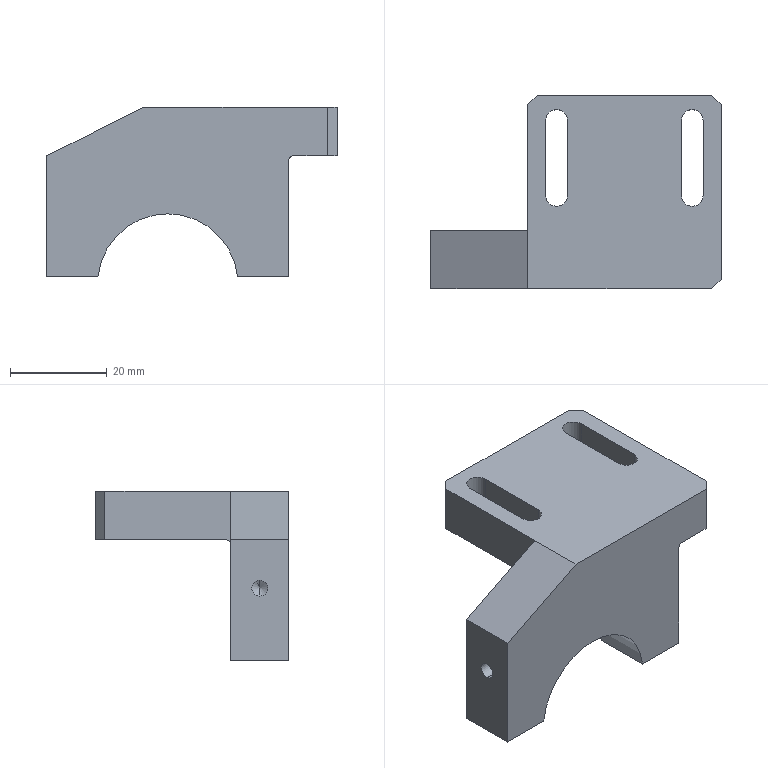Part | 1 solid | 52 faces | box 60 x 40 x 35 mm | volume 25774 mm3 | plane 25 | cylinder 19 | cone 8 | commonest cylinder face diameters 3.3 x8 4.5 x4 8 x4 2 x2 29 x1
STEP:
#1=CARTESIAN_POINT('',(-28.5,-14.,-21.65));
#2=VERTEX_POINT('',#1);
#3=CARTESIAN_POINT('',(-28.5,-14.,-18.35));
#4=VERTEX_POINT('',#3);
#5=CARTESIAN_POINT('',(-28.5,-14.,-20.));
#6=DIRECTION('',(-1.,0.,0.));
#7=DIRECTION('',(0.,0.,1.));
#8=AXIS2_PLACEMENT_3D('',#5,#6,#7);
#9=CIRCLE('',#8,1.65);
#10=EDGE_CURVE('',#2,#4,#9,.T.);
#11=ORIENTED_EDGE('',*,*,#10,.F.);
#12=CARTESIAN_POINT('',(-40.,-14.,-21.65));
#13=VERTEX_POINT('',#12);
#14=CARTESIAN_POINT('',(-40.,-14.,-21.65));
#15=DIRECTION('',(-1.,0.,0.));
#16=VECTOR('',#15,1000.);
#17=LINE('',#14,#16);
#18=EDGE_CURVE('',#13,#2,#17,.F.);
#19=ORIENTED_EDGE('',*,*,#18,.F.);
#20=CARTESIAN_POINT('',(-40.,-14.,-18.35));
#21=VERTEX_POINT('',#20);
#22=CARTESIAN_POINT('',(-40.,-14.,-20.));
#23=DIRECTION('',(-1.,0.,0.));
#24=DIRECTION('',(0.,0.,1.));
#25=AXIS2_PLACEMENT_3D('',#22,#23,#24);
#26=CIRCLE('',#25,1.65);
#27=EDGE_CURVE('',#13,#21,#26,.T.);
#28=ORIENTED_EDGE('',*,*,#27,.T.);
#29=CARTESIAN_POINT('',(-40.,-14.,-18.35));
#30=DIRECTION('',(-1.,0.,0.));
#31=VECTOR('',#30,1000.);
#32=LINE('',#29,#31);
#33=EDGE_CURVE('',#21,#4,#32,.F.);
#34=ORIENTED_EDGE('',*,*,#33,.T.);
#35=EDGE_LOOP('',(#11,#19,#28,#34));
#36=FACE_BOUND('',#35,.T.);
#37=CARTESIAN_POINT('',(-40.,-14.,-20.));
#38=DIRECTION('',(-1.,0.,0.));
#39=DIRECTION('',(0.,0.,-1.));
#40=AXIS2_PLACEMENT_3D('',#37,#38,#39);
#41=CYLINDRICAL_SURFACE('',#40,1.65);
#42=ADVANCED_FACE('',(#36),#41,.F.);
#43=CARTESIAN_POINT('',(-27.509,-14.,-20.));
#44=VERTEX_POINT('',#43);
#45=CARTESIAN_POINT('',(-28.5,-14.,-18.35));
#46=DIRECTION('',(-0.515,0.,0.8572));
#47=VECTOR('',#46,1000.);
#48=LINE('',#45,#47);
#49=EDGE_CURVE('',#4,#44,#48,.F.);
#50=ORIENTED_EDGE('',*,*,#49,.T.);
#51=CARTESIAN_POINT('',(-28.5,-14.,-21.65));
#52=DIRECTION('',(-0.515,0.,-0.8572));
#53=VECTOR('',#52,1000.);
#54=LINE('',#51,#53);
#55=EDGE_CURVE('',#2,#44,#54,.F.);
#56=ORIENTED_EDGE('',*,*,#55,.F.);
#57=ORIENTED_EDGE('',*,*,#10,.T.);
#58=EDGE_LOOP('',(#50,#56,#57));
#59=FACE_BOUND('',#58,.T.);
#60=CARTESIAN_POINT('',(-28.5,-14.,-20.));
#61=DIRECTION('',(-1.,0.,0.));
#62=DIRECTION('',(0.,0.,-1.));
#63=AXIS2_PLACEMENT_3D('',#60,#61,#62);
#64=CONICAL_SURFACE('',#63,1.65,1.03);
#65=ADVANCED_FACE('',(#59),#64,.F.);
#66=CARTESIAN_POINT('',(-1.5,-14.,-18.35));
#67=VERTEX_POINT('',#66);
#68=CARTESIAN_POINT('',(-1.5,-14.,-21.65));
#69=VERTEX_POINT('',#68);
#70=CARTESIAN_POINT('',(-1.5,-14.,-20.));
#71=DIRECTION('',(1.,0.,0.));
#72=DIRECTION('',(0.,0.,-1.));
#73=AXIS2_PLACEMENT_3D('',#70,#71,#72);
#74=CIRCLE('',#73,1.65);
#75=EDGE_CURVE('',#67,#69,#74,.T.);
#76=ORIENTED_EDGE('',*,*,#75,.F.);
#77=CARTESIAN_POINT('',(10.,-14.,-18.35));
#78=VERTEX_POINT('',#77);
#79=CARTESIAN_POINT('',(10.,-14.,-18.35));
#80=DIRECTION('',(1.,0.,0.));
#81=VECTOR('',#80,1000.);
#82=LINE('',#79,#81);
#83=EDGE_CURVE('',#78,#67,#82,.F.);
#84=ORIENTED_EDGE('',*,*,#83,.F.);
#85=CARTESIAN_POINT('',(10.,-14.,-21.65));
#86=VERTEX_POINT('',#85);
#87=CARTESIAN_POINT('',(10.,-14.,-20.));
#88=DIRECTION('',(1.,0.,0.));
#89=DIRECTION('',(0.,0.,-1.));
#90=AXIS2_PLACEMENT_3D('',#87,#88,#89);
#91=CIRCLE('',#90,1.65);
#92=EDGE_CURVE('',#78,#86,#91,.T.);
#93=ORIENTED_EDGE('',*,*,#92,.T.);
#94=CARTESIAN_POINT('',(10.,-14.,-21.65));
#95=DIRECTION('',(1.,0.,0.));
#96=VECTOR('',#95,1000.);
#97=LINE('',#94,#96);
#98=EDGE_CURVE('',#86,#69,#97,.F.);
#99=ORIENTED_EDGE('',*,*,#98,.T.);
#100=EDGE_LOOP('',(#76,#84,#93,#99));
#101=FACE_BOUND('',#100,.T.);
#102=CARTESIAN_POINT('',(10.,-14.,-20.));
#103=DIRECTION('',(1.,0.,0.));
#104=DIRECTION('',(0.,0.,1.));
#105=AXIS2_PLACEMENT_3D('',#102,#103,#104);
#106=CYLINDRICAL_SURFACE('',#105,1.65);
#107=ADVANCED_FACE('',(#101),#106,.F.);
#108=CARTESIAN_POINT('',(-2.491,-14.,-20.));
#109=VERTEX_POINT('',#108);
#110=CARTESIAN_POINT('',(-1.5,-14.,-21.65));
#111=DIRECTION('',(0.515,0.,-0.8572));
#112=VECTOR('',#111,1000.);
#113=LINE('',#110,#112);
#114=EDGE_CURVE('',#69,#109,#113,.F.);
#115=ORIENTED_EDGE('',*,*,#114,.T.);
#116=CARTESIAN_POINT('',(-1.5,-14.,-18.35));
#117=DIRECTION('',(0.515,0.,0.8572));
#118=VECTOR('',#117,1000.);
#119=LINE('',#116,#118);
#120=EDGE_CURVE('',#67,#109,#119,.F.);
#121=ORIENTED_EDGE('',*,*,#120,.F.);
#122=ORIENTED_EDGE('',*,*,#75,.T.);
#123=EDGE_LOOP('',(#115,#121,#122));
#124=FACE_BOUND('',#123,.T.);
#125=CARTESIAN_POINT('',(-1.5,-14.,-20.));
#126=DIRECTION('',(1.,0.,0.));
#127=DIRECTION('',(0.,0.,1.));
#128=AXIS2_PLACEMENT_3D('',#125,#126,#127);
#129=CONICAL_SURFACE('',#128,1.65,1.03);
#130=ADVANCED_FACE('',(#124),#129,.F.);
#131=CARTESIAN_POINT('',(6.65,-14.,-23.5));
#132=VERTEX_POINT('',#131);
#133=CARTESIAN_POINT('',(3.35,-14.,-23.5));
#134=VERTEX_POINT('',#133);
#135=CARTESIAN_POINT('',(5.,-14.,-23.5));
#136=DIRECTION('',(0.,0.,-1.));
#137=DIRECTION('',(-1.,0.,0.));
#138=AXIS2_PLACEMENT_3D('',#135,#136,#137);
#139=CIRCLE('',#138,1.65);
#140=EDGE_CURVE('',#132,#134,#139,.T.);
#141=ORIENTED_EDGE('',*,*,#140,.F.);
#142=CARTESIAN_POINT('',(6.65,-14.,-35.));
#143=VERTEX_POINT('',#142);
#144=CARTESIAN_POINT('',(6.65,-14.,-35.));
#145=DIRECTION('',(0.,0.,-1.));
#146=VECTOR('',#145,1000.);
#147=LINE('',#144,#146);
#148=EDGE_CURVE('',#143,#132,#147,.F.);
#149=ORIENTED_EDGE('',*,*,#148,.F.);
#150=CARTESIAN_POINT('',(3.35,-14.,-35.));
#151=VERTEX_POINT('',#150);
#152=CARTESIAN_POINT('',(5.,-14.,-35.));
#153=DIRECTION('',(0.,0.,-1.));
#154=DIRECTION('',(-1.,0.,0.));
#155=AXIS2_PLACEMENT_3D('',#152,#153,#154);
#156=CIRCLE('',#155,1.65);
#157=EDGE_CURVE('',#143,#151,#156,.T.);
#158=ORIENTED_EDGE('',*,*,#157,.T.);
#159=CARTESIAN_POINT('',(3.35,-14.,-35.));
#160=DIRECTION('',(0.,0.,-1.));
#161=VECTOR('',#160,1000.);
#162=LINE('',#159,#161);
#163=EDGE_CURVE('',#151,#134,#162,.F.);
#164=ORIENTED_EDGE('',*,*,#163,.T.);
#165=EDGE_LOOP('',(#141,#149,#158,#164));
#166=FACE_BOUND('',#165,.T.);
#167=CARTESIAN_POINT('',(5.,-14.,-35.));
#168=DIRECTION('',(0.,0.,-1.));
#169=DIRECTION('',(1.,0.,0.));
#170=AXIS2_PLACEMENT_3D('',#167,#168,#169);
#171=CYLINDRICAL_SURFACE('',#170,1.65);
#172=ADVANCED_FACE('',(#166),#171,.F.);
#173=CARTESIAN_POINT('',(5.,-14.,-22.509));
#174=VERTEX_POINT('',#173);
#175=CARTESIAN_POINT('',(3.35,-14.,-23.5));
#176=DIRECTION('',(-0.8572,0.,-0.515));
#177=VECTOR('',#176,1000.);
#178=LINE('',#175,#177);
#179=EDGE_CURVE('',#134,#174,#178,.F.);
#180=ORIENTED_EDGE('',*,*,#179,.T.);
#181=CARTESIAN_POINT('',(6.65,-14.,-23.5));
#182=DIRECTION('',(0.8572,0.,-0.515));
#183=VECTOR('',#182,1000.);
#184=LINE('',#181,#183);
#185=EDGE_CURVE('',#132,#174,#184,.F.);
#186=ORIENTED_EDGE('',*,*,#185,.F.);
#187=ORIENTED_EDGE('',*,*,#140,.T.);
#188=EDGE_LOOP('',(#180,#186,#187));
#189=FACE_BOUND('',#188,.T.);
#190=CARTESIAN_POINT('',(5.,-14.,-23.5));
#191=DIRECTION('',(0.,0.,-1.));
#192=DIRECTION('',(1.,0.,0.));
#193=AXIS2_PLACEMENT_3D('',#190,#191,#192);
#194=CONICAL_SURFACE('',#193,1.65,1.03);
#195=ADVANCED_FACE('',(#189),#194,.F.);
#196=CARTESIAN_POINT('',(-33.35,-14.,-23.5));
#197=VERTEX_POINT('',#196);
#198=CARTESIAN_POINT('',(-36.65,-14.,-23.5));
#199=VERTEX_POINT('',#198);
#200=CARTESIAN_POINT('',(-35.,-14.,-23.5));
#201=DIRECTION('',(0.,0.,-1.));
#202=DIRECTION('',(-1.,0.,0.));
#203=AXIS2_PLACEMENT_3D('',#200,#201,#202);
#204=CIRCLE('',#203,1.65);
#205=EDGE_CURVE('',#197,#199,#204,.T.);
#206=ORIENTED_EDGE('',*,*,#205,.F.);
#207=CARTESIAN_POINT('',(-33.35,-14.,-35.));
#208=VERTEX_POINT('',#207);
#209=CARTESIAN_POINT('',(-33.35,-14.,-35.));
#210=DIRECTION('',(0.,0.,-1.));
#211=VECTOR('',#210,1000.);
#212=LINE('',#209,#211);
#213=EDGE_CURVE('',#208,#197,#212,.F.);
#214=ORIENTED_EDGE('',*,*,#213,.F.);
#215=CARTESIAN_POINT('',(-36.65,-14.,-35.));
#216=VERTEX_POINT('',#215);
#217=CARTESIAN_POINT('',(-35.,-14.,-35.));
#218=DIRECTION('',(0.,0.,-1.));
#219=DIRECTION('',(-1.,0.,0.));
#220=AXIS2_PLACEMENT_3D('',#217,#218,#219);
#221=CIRCLE('',#220,1.65);
#222=EDGE_CURVE('',#208,#216,#221,.T.);
#223=ORIENTED_EDGE('',*,*,#222,.T.);
#224=CARTESIAN_POINT('',(-36.65,-14.,-35.));
#225=DIRECTION('',(0.,0.,-1.));
#226=VECTOR('',#225,1000.);
#227=LINE('',#224,#226);
#228=EDGE_CURVE('',#216,#199,#227,.F.);
#229=ORIENTED_EDGE('',*,*,#228,.T.);
#230=EDGE_LOOP('',(#206,#214,#223,#229));
#231=FACE_BOUND('',#230,.T.);
#232=CARTESIAN_POINT('',(-35.,-14.,-35.));
#233=DIRECTION('',(0.,0.,-1.));
#234=DIRECTION('',(1.,0.,0.));
#235=AXIS2_PLACEMENT_3D('',#232,#233,#234);
#236=CYLINDRICAL_SURFACE('',#235,1.65);
#237=ADVANCED_FACE('',(#231),#236,.F.);
#238=CARTESIAN_POINT('',(-35.,-14.,-22.509));
#239=VERTEX_POINT('',#238);
#240=CARTESIAN_POINT('',(-36.65,-14.,-23.5));
#241=DIRECTION('',(-0.8572,0.,-0.515));
#242=VECTOR('',#241,1000.);
#243=LINE('',#240,#242);
#244=EDGE_CURVE('',#199,#239,#243,.F.);
#245=ORIENTED_EDGE('',*,*,#244,.T.);
#246=CARTESIAN_POINT('',(-33.35,-14.,-23.5));
#247=DIRECTION('',(0.8572,0.,-0.515));
#248=VECTOR('',#247,1000.);
#249=LINE('',#246,#248);
#250=EDGE_CURVE('',#197,#239,#249,.F.);
#251=ORIENTED_EDGE('',*,*,#250,.F.);
#252=ORIENTED_EDGE('',*,*,#205,.T.);
#253=EDGE_LOOP('',(#245,#251,#252));
#254=FACE_BOUND('',#253,.T.);
#255=CARTESIAN_POINT('',(-35.,-14.,-23.5));
#256=DIRECTION('',(0.,0.,-1.));
#257=DIRECTION('',(1.,0.,0.));
#258=AXIS2_PLACEMENT_3D('',#255,#256,#257);
#259=CONICAL_SURFACE('',#258,1.65,1.03);
#260=ADVANCED_FACE('',(#254),#259,.F.);
#261=CARTESIAN_POINT('',(18.,-0.75,-10.));
#262=VERTEX_POINT('',#261);
#263=CARTESIAN_POINT('',(18.,14.75,-10.));
#264=VERTEX_POINT('',#263);
#265=CARTESIAN_POINT('',(18.,-0.75,-10.));
#266=DIRECTION('',(0.,1.,0.));
#267=VECTOR('',#266,1000.);
#268=LINE('',#265,#267);
#269=EDGE_CURVE('',#262,#264,#268,.T.);
#270=ORIENTED_EDGE('',*,*,#269,.T.);
#271=CARTESIAN_POINT('',(10.,14.75,-10.));
#272=VERTEX_POINT('',#271);
#273=CARTESIAN_POINT('',(14.,14.75,-10.));
#274=DIRECTION('',(0.,0.,-1.));
#275=DIRECTION('',(-1.,0.,0.));
#276=AXIS2_PLACEMENT_3D('',#273,#274,#275);
#277=CIRCLE('',#276,4.);
#278=EDGE_CURVE('',#272,#264,#277,.T.);
#279=ORIENTED_EDGE('',*,*,#278,.F.);
#280=CARTESIAN_POINT('',(10.,-0.75,-10.));
#281=VERTEX_POINT('',#280);
#282=CARTESIAN_POINT('',(10.,-0.75,-10.));
#283=DIRECTION('',(0.,1.,0.));
#284=VECTOR('',#283,1000.);
#285=LINE('',#282,#284);
#286=EDGE_CURVE('',#281,#272,#285,.T.);
#287=ORIENTED_EDGE('',*,*,#286,.F.);
#288=CARTESIAN_POINT('',(14.,-0.75,-10.));
#289=DIRECTION('',(0.,0.,-1.));
#290=DIRECTION('',(-1.,0.,0.));
#291=AXIS2_PLACEMENT_3D('',#288,#289,#290);
#292=CIRCLE('',#291,4.);
#293=EDGE_CURVE('',#262,#281,#292,.T.);
#294=ORIENTED_EDGE('',*,*,#293,.F.);
#295=EDGE_LOOP('',(#270,#279,#287,#294));
#296=FACE_BOUND('',#295,.T.);
#297=CARTESIAN_POINT('',(11.,-20.,-10.));
#298=VERTEX_POINT('',#297);
#299=CARTESIAN_POINT('',(18.,-20.,-10.));
#300=VERTEX_POINT('',#299);
#301=CARTESIAN_POINT('',(-40.,-20.,-10.));
#302=DIRECTION('',(1.,0.,0.));
#303=VECTOR('',#302,1000.);
#304=LINE('',#301,#303);
#305=EDGE_CURVE('',#298,#300,#304,.T.);
#306=ORIENTED_EDGE('',*,*,#305,.F.);
#307=CARTESIAN_POINT('',(11.,-7.,-10.));
#308=VERTEX_POINT('',#307);
#309=CARTESIAN_POINT('',(11.,-8.,-10.));
#310=DIRECTION('',(0.,1.,0.));
#311=VECTOR('',#310,1000.);
#312=LINE('',#309,#311);
#313=EDGE_CURVE('',#298,#308,#312,.T.);
#314=ORIENTED_EDGE('',*,*,#313,.T.);
#315=CARTESIAN_POINT('',(-20.,-7.,-10.));
#316=VERTEX_POINT('',#315);
#317=CARTESIAN_POINT('',(-20.,-7.,-10.));
#318=DIRECTION('',(-1.,0.,0.));
#319=VECTOR('',#318,1000.);
#320=LINE('',#317,#319);
#321=EDGE_CURVE('',#308,#316,#320,.T.);
#322=ORIENTED_EDGE('',*,*,#321,.T.);
#323=CARTESIAN_POINT('',(-20.,18.,-10.));
#324=VERTEX_POINT('',#323);
#325=CARTESIAN_POINT('',(-20.,20.,-10.));
#326=DIRECTION('',(0.,1.,0.));
#327=VECTOR('',#326,1000.);
#328=LINE('',#325,#327);
#329=EDGE_CURVE('',#316,#324,#328,.T.);
#330=ORIENTED_EDGE('',*,*,#329,.T.);
#331=CARTESIAN_POINT('',(-18.,20.,-10.));
#332=VERTEX_POINT('',#331);
#333=CARTESIAN_POINT('',(-20.,18.,-10.));
#334=DIRECTION('',(0.7071,0.7071,0.));
#335=VECTOR('',#334,1000.);
#336=LINE('',#333,#335);
#337=EDGE_CURVE('',#324,#332,#336,.T.);
#338=ORIENTED_EDGE('',*,*,#337,.T.);
#339=CARTESIAN_POINT('',(18.,20.,-10.));
#340=VERTEX_POINT('',#339);
#341=CARTESIAN_POINT('',(-40.001,20.,-10.));
#342=DIRECTION('',(1.,0.,0.));
#343=VECTOR('',#342,1000.);
#344=LINE('',#341,#343);
#345=EDGE_CURVE('',#332,#340,#344,.T.);
#346=ORIENTED_EDGE('',*,*,#345,.T.);
#347=CARTESIAN_POINT('',(20.,18.,-10.));
#348=VERTEX_POINT('',#347);
#349=CARTESIAN_POINT('',(20.,18.,-10.));
#350=DIRECTION('',(0.7071,-0.7071,0.));
#351=VECTOR('',#350,1000.);
#352=LINE('',#349,#351);
#353=EDGE_CURVE('',#340,#348,#352,.T.);
#354=ORIENTED_EDGE('',*,*,#353,.T.);
#355=CARTESIAN_POINT('',(20.,-18.,-10.));
#356=VERTEX_POINT('',#355);
#357=CARTESIAN_POINT('',(20.,20.,-10.));
#358=DIRECTION('',(0.,-1.,0.));
#359=VECTOR('',#358,1000.);
#360=LINE('',#357,#359);
#361=EDGE_CURVE('',#348,#356,#360,.T.);
#362=ORIENTED_EDGE('',*,*,#361,.T.);
#363=CARTESIAN_POINT('',(18.,-20.,-10.));
#364=DIRECTION('',(-0.7071,-0.7071,0.));
#365=VECTOR('',#364,1000.);
#366=LINE('',#363,#365);
#367=EDGE_CURVE('',#356,#300,#366,.T.);
#368=ORIENTED_EDGE('',*,*,#367,.T.);
#369=EDGE_LOOP('',(#306,#314,#322,#330,#338,#346,#354,#362,#368));
#370=FACE_BOUND('',#369,.T.);
#371=CARTESIAN_POINT('',(-18.,14.75,-10.));
#372=VERTEX_POINT('',#371);
#373=CARTESIAN_POINT('',(-10.,14.75,-10.));
#374=VERTEX_POINT('',#373);
#375=CARTESIAN_POINT('',(-14.,14.75,-10.));
#376=DIRECTION('',(0.,0.,-1.));
#377=DIRECTION('',(-1.,0.,0.));
#378=AXIS2_PLACEMENT_3D('',#375,#376,#377);
#379=CIRCLE('',#378,4.);
#380=EDGE_CURVE('',#372,#374,#379,.T.);
#381=ORIENTED_EDGE('',*,*,#380,.F.);
#382=CARTESIAN_POINT('',(-18.,-0.75,-10.));
#383=VERTEX_POINT('',#382);
#384=CARTESIAN_POINT('',(-18.,-0.75,-10.));
#385=DIRECTION('',(0.,1.,0.));
#386=VECTOR('',#385,1000.);
#387=LINE('',#384,#386);
#388=EDGE_CURVE('',#383,#372,#387,.T.);
#389=ORIENTED_EDGE('',*,*,#388,.F.);
#390=CARTESIAN_POINT('',(-10.,-0.75,-10.));
#391=VERTEX_POINT('',#390);
#392=CARTESIAN_POINT('',(-14.,-0.75,-10.));
#393=DIRECTION('',(0.,0.,-1.));
#394=DIRECTION('',(-1.,0.,0.));
#395=AXIS2_PLACEMENT_3D('',#392,#393,#394);
#396=CIRCLE('',#395,4.);
#397=EDGE_CURVE('',#391,#383,#396,.T.);
#398=ORIENTED_EDGE('',*,*,#397,.F.);
#399=CARTESIAN_POINT('',(-10.,-0.75,-10.));
#400=DIRECTION('',(0.,1.,0.));
#401=VECTOR('',#400,1000.);
#402=LINE('',#399,#401);
#403=EDGE_CURVE('',#391,#374,#402,.T.);
#404=ORIENTED_EDGE('',*,*,#403,.T.);
#405=EDGE_LOOP('',(#381,#389,#398,#404));
#406=FACE_BOUND('',#405,.T.);
#407=CARTESIAN_POINT('',(-40.001,20.,-10.));
#408=DIRECTION('',(0.,0.,1.));
#409=DIRECTION('',(0.,-1.,0.));
#410=AXIS2_PLACEMENT_3D('',#407,#408,#409);
#411=PLANE('',#410);
#412=ADVANCED_FACE('',(#296,#370,#406),#411,.F.);
#413=ORIENTED_EDGE('',*,*,#329,.F.);
#414=CARTESIAN_POINT('',(-20.,-8.,-11.));
#415=VERTEX_POINT('',#414);
#416=CARTESIAN_POINT('',(-20.,-7.,-11.));
#417=DIRECTION('',(1.,0.,0.));
#418=DIRECTION('',(0.,1.,0.));
#419=AXIS2_PLACEMENT_3D('',#416,#417,#418);
#420=CIRCLE('',#419,1.);
#421=EDGE_CURVE('',#316,#415,#420,.T.);
#422=ORIENTED_EDGE('',*,*,#421,.T.);
#423=CARTESIAN_POINT('',(-20.,-8.,0.));
#424=VERTEX_POINT('',#423);
#425=CARTESIAN_POINT('',(-20.,-8.,0.));
#426=DIRECTION('',(0.,0.,-1.));
#427=VECTOR('',#426,1000.);
#428=LINE('',#425,#427);
#429=EDGE_CURVE('',#424,#415,#428,.T.);
#430=ORIENTED_EDGE('',*,*,#429,.F.);
#431=CARTESIAN_POINT('',(-20.,18.,0.));
#432=VERTEX_POINT('',#431);
#433=CARTESIAN_POINT('',(-20.,20.,0.));
#434=DIRECTION('',(0.,-1.,0.));
#435=VECTOR('',#434,1000.);
#436=LINE('',#433,#435);
#437=EDGE_CURVE('',#432,#424,#436,.T.);
#438=ORIENTED_EDGE('',*,*,#437,.F.);
#439=CARTESIAN_POINT('',(-20.,18.,0.));
#440=DIRECTION('',(0.,0.,-1.));
#441=VECTOR('',#440,1000.);
#442=LINE('',#439,#441);
#443=EDGE_CURVE('',#432,#324,#442,.T.);
#444=ORIENTED_EDGE('',*,*,#443,.T.);
#445=EDGE_LOOP('',(#413,#422,#430,#438,#444));
#446=FACE_BOUND('',#445,.T.);
#447=CARTESIAN_POINT('',(-20.,20.,0.));
#448=DIRECTION('',(1.,0.,0.));
#449=DIRECTION('',(0.,1.,0.));
#450=AXIS2_PLACEMENT_3D('',#447,#448,#449);
#451=PLANE('',#450);
#452=ADVANCED_FACE('',(#446),#451,.F.);
#453=CARTESIAN_POINT('',(-35.,-14.,-35.));
#454=DIRECTION('',(0.,0.,-1.));
#455=DIRECTION('',(-1.,0.,0.));
#456=AXIS2_PLACEMENT_3D('',#453,#454,#455);
#457=CIRCLE('',#456,1.65);
#458=EDGE_CURVE('',#216,#208,#457,.T.);
#459=ORIENTED_EDGE('',*,*,#458,.F.);
#460=ORIENTED_EDGE('',*,*,#222,.F.);
#461=EDGE_LOOP('',(#459,#460));
#462=FACE_BOUND('',#461,.T.);
#463=CARTESIAN_POINT('',(-40.,-8.,-35.));
#464=VERTEX_POINT('',#463);
#465=CARTESIAN_POINT('',(-29.422,-8.,-35.));
#466=VERTEX_POINT('',#465);
#467=CARTESIAN_POINT('',(-40.001,-8.,-35.));
#468=DIRECTION('',(1.,0.,0.));
#469=VECTOR('',#468,1000.);
#470=LINE('',#467,#469);
#471=EDGE_CURVE('',#464,#466,#470,.T.);
#472=ORIENTED_EDGE('',*,*,#471,.T.);
#473=CARTESIAN_POINT('',(-29.422,-20.,-35.));
#474=VERTEX_POINT('',#473);
#475=CARTESIAN_POINT('',(-29.422,20.001,-35.));
#476=DIRECTION('',(0.,1.,0.));
#477=VECTOR('',#476,1000.);
#478=LINE('',#475,#477);
#479=EDGE_CURVE('',#474,#466,#478,.T.);
#480=ORIENTED_EDGE('',*,*,#479,.F.);
#481=CARTESIAN_POINT('',(-40.,-20.,-35.));
#482=VERTEX_POINT('',#481);
#483=CARTESIAN_POINT('',(-40.,-20.,-35.));
#484=DIRECTION('',(-1.,0.,0.));
#485=VECTOR('',#484,1000.);
#486=LINE('',#483,#485);
#487=EDGE_CURVE('',#474,#482,#486,.T.);
#488=ORIENTED_EDGE('',*,*,#487,.T.);
#489=CARTESIAN_POINT('',(-40.,20.,-35.));
#490=DIRECTION('',(0.,1.,0.));
#491=VECTOR('',#490,1000.);
#492=LINE('',#489,#491);
#493=EDGE_CURVE('',#482,#464,#492,.T.);
#494=ORIENTED_EDGE('',*,*,#493,.T.);
#495=EDGE_LOOP('',(#472,#480,#488,#494));
#496=FACE_BOUND('',#495,.T.);
#497=CARTESIAN_POINT('',(-10.,0.,-35.));
#498=DIRECTION('',(0.,0.,1.));
#499=DIRECTION('',(-1.,0.,0.));
#500=AXIS2_PLACEMENT_3D('',#497,#498,#499);
#501=PLANE('',#500);
#502=ADVANCED_FACE('',(#462,#496),#501,.F.);
#503=ORIENTED_EDGE('',*,*,#361,.F.);
#504=CARTESIAN_POINT('',(20.,18.,0.));
#505=VERTEX_POINT('',#504);
#506=CARTESIAN_POINT('',(20.,18.,-35.));
#507=DIRECTION('',(0.,0.,1.));
#508=VECTOR('',#507,1000.);
#509=LINE('',#506,#508);
#510=EDGE_CURVE('',#348,#505,#509,.T.);
#511=ORIENTED_EDGE('',*,*,#510,.T.);
#512=CARTESIAN_POINT('',(20.,-18.,0.));
#513=VERTEX_POINT('',#512);
#514=CARTESIAN_POINT('',(20.,20.,0.));
#515=DIRECTION('',(0.,-1.,0.));
#516=VECTOR('',#515,1000.);
#517=LINE('',#514,#516);
#518=EDGE_CURVE('',#505,#513,#517,.T.);
#519=ORIENTED_EDGE('',*,*,#518,.T.);
#520=CARTESIAN_POINT('',(20.,-18.,-35.));
#521=DIRECTION('',(0.,0.,-1.));
#522=VECTOR('',#521,1000.);
#523=LINE('',#520,#522);
#524=EDGE_CURVE('',#513,#356,#523,.T.);
#525=ORIENTED_EDGE('',*,*,#524,.T.);
#526=EDGE_LOOP('',(#503,#511,#519,#525));
#527=FACE_BOUND('',#526,.T.);
#528=CARTESIAN_POINT('',(20.,20.,-35.));
#529=DIRECTION('',(-1.,0.,0.));
#530=DIRECTION('',(0.,-1.,0.));
#531=AXIS2_PLACEMENT_3D('',#528,#529,#530);
#532=PLANE('',#531);
#533=ADVANCED_FACE('',(#527),#532,.F.);
#534=CARTESIAN_POINT('',(18.,-20.,0.));
#535=VERTEX_POINT('',#534);
#536=CARTESIAN_POINT('',(-20.,-20.,0.));
#537=VERTEX_POINT('',#536);
#538=CARTESIAN_POINT('',(-40.,-20.,0.));
#539=DIRECTION('',(-1.,0.,0.));
#540=VECTOR('',#539,1000.);
#541=LINE('',#538,#540);
#542=EDGE_CURVE('',#535,#537,#541,.T.);
#543=ORIENTED_EDGE('',*,*,#542,.T.);
#544=CARTESIAN_POINT('',(-40.,-20.,-10.));
#545=VERTEX_POINT('',#544);
#546=CARTESIAN_POINT('',(-40.,-20.,-10.));
#547=DIRECTION('',(-0.8944,0.,-0.4472));
#548=VECTOR('',#547,1000.);
#549=LINE('',#546,#548);
#550=EDGE_CURVE('',#537,#545,#549,.T.);
#551=ORIENTED_EDGE('',*,*,#550,.T.);
#552=CARTESIAN_POINT('',(-40.,-20.,-35.));
#553=DIRECTION('',(0.,0.,1.));
#554=VECTOR('',#553,1000.);
#555=LINE('',#552,#554);
#556=EDGE_CURVE('',#482,#545,#555,.T.);
#557=ORIENTED_EDGE('',*,*,#556,.F.);
#558=ORIENTED_EDGE('',*,*,#487,.F.);
#559=CARTESIAN_POINT('',(-0.5778,-20.,-35.));
#560=VERTEX_POINT('',#559);
#561=CARTESIAN_POINT('',(-15.,-20.,-36.5));
#562=DIRECTION('',(0.,-1.,0.));
#563=DIRECTION('',(-1.,0.,0.));
#564=AXIS2_PLACEMENT_3D('',#561,#562,#563);
#565=CIRCLE('',#564,14.5);
#566=EDGE_CURVE('',#560,#474,#565,.T.);
#567=ORIENTED_EDGE('',*,*,#566,.F.);
#568=CARTESIAN_POINT('',(10.,-20.,-35.));
#569=VERTEX_POINT('',#568);
#570=CARTESIAN_POINT('',(-40.,-20.,-35.));
#571=DIRECTION('',(-1.,0.,0.));
#572=VECTOR('',#571,1000.);
#573=LINE('',#570,#572);
#574=EDGE_CURVE('',#569,#560,#573,.T.);
#575=ORIENTED_EDGE('',*,*,#574,.F.);
#576=CARTESIAN_POINT('',(10.,-20.,-11.));
#577=VERTEX_POINT('',#576);
#578=CARTESIAN_POINT('',(10.,-20.,-35.));
#579=DIRECTION('',(0.,0.,1.));
#580=VECTOR('',#579,1000.);
#581=LINE('',#578,#580);
#582=EDGE_CURVE('',#569,#577,#581,.T.);
#583=ORIENTED_EDGE('',*,*,#582,.T.);
#584=CARTESIAN_POINT('',(11.,-20.,-11.));
#585=DIRECTION('',(0.,1.,0.));
#586=DIRECTION('',(1.,0.,0.));
#587=AXIS2_PLACEMENT_3D('',#584,#585,#586);
#588=CIRCLE('',#587,1.);
#589=EDGE_CURVE('',#577,#298,#588,.T.);
#590=ORIENTED_EDGE('',*,*,#589,.T.);
#591=ORIENTED_EDGE('',*,*,#305,.T.);
#592=CARTESIAN_POINT('',(18.,-20.,-35.));
#593=DIRECTION('',(0.,0.,1.));
#594=VECTOR('',#593,1000.);
#595=LINE('',#592,#594);
#596=EDGE_CURVE('',#300,#535,#595,.T.);
#597=ORIENTED_EDGE('',*,*,#596,.T.);
#598=EDGE_LOOP('',(#543,#551,#557,#558,#567,#575,#583,#590,#591,#597));
#599=FACE_BOUND('',#598,.T.);
#600=CARTESIAN_POINT('',(-40.,-20.,-35.));
#601=DIRECTION('',(0.,1.,0.));
#602=DIRECTION('',(-1.,0.,0.));
#603=AXIS2_PLACEMENT_3D('',#600,#601,#602);
#604=PLANE('',#603);
#605=ADVANCED_FACE('',(#599),#604,.F.);
#606=CARTESIAN_POINT('',(-40.,-14.,-20.));
#607=DIRECTION('',(-1.,0.,0.));
#608=DIRECTION('',(0.,0.,1.));
#609=AXIS2_PLACEMENT_3D('',#606,#607,#608);
#610=CIRCLE('',#609,1.65);
#611=EDGE_CURVE('',#21,#13,#610,.T.);
#612=ORIENTED_EDGE('',*,*,#611,.F.);
#613=ORIENTED_EDGE('',*,*,#27,.F.);
#614=EDGE_LOOP('',(#612,#613));
#615=FACE_BOUND('',#614,.T.);
#616=ORIENTED_EDGE('',*,*,#556,.T.);
#617=CARTESIAN_POINT('',(-40.,-8.,-10.));
#618=VERTEX_POINT('',#617);
#619=CARTESIAN_POINT('',(-40.,-20.001,-10.));
#620=DIRECTION('',(0.,1.,0.));
#621=VECTOR('',#620,1000.);
#622=LINE('',#619,#621);
#623=EDGE_CURVE('',#545,#618,#622,.T.);
#624=ORIENTED_EDGE('',*,*,#623,.T.);
#625=CARTESIAN_POINT('',(-40.,-8.,-35.));
#626=DIRECTION('',(0.,0.,1.));
#627=VECTOR('',#626,1000.);
#628=LINE('',#625,#627);
#629=EDGE_CURVE('',#464,#618,#628,.T.);
#630=ORIENTED_EDGE('',*,*,#629,.F.);
#631=ORIENTED_EDGE('',*,*,#493,.F.);
#632=EDGE_LOOP('',(#616,#624,#630,#631));
#633=FACE_BOUND('',#632,.T.);
#634=CARTESIAN_POINT('',(-40.,20.,-35.));
#635=DIRECTION('',(1.,0.,0.));
#636=DIRECTION('',(0.,1.,0.));
#637=AXIS2_PLACEMENT_3D('',#634,#635,#636);
#638=PLANE('',#637);
#639=ADVANCED_FACE('',(#615,#633),#638,.F.);
#640=ORIENTED_EDGE('',*,*,#345,.F.);
#641=CARTESIAN_POINT('',(-18.,20.,0.));
#642=VERTEX_POINT('',#641);
#643=CARTESIAN_POINT('',(-18.,20.,-35.));
#644=DIRECTION('',(0.,0.,1.));
#645=VECTOR('',#644,1000.);
#646=LINE('',#643,#645);
#647=EDGE_CURVE('',#332,#642,#646,.T.);
#648=ORIENTED_EDGE('',*,*,#647,.T.);
#649=CARTESIAN_POINT('',(18.,20.,0.));
#650=VERTEX_POINT('',#649);
#651=CARTESIAN_POINT('',(-40.,20.,0.));
#652=DIRECTION('',(1.,0.,0.));
#653=VECTOR('',#652,1000.);
#654=LINE('',#651,#653);
#655=EDGE_CURVE('',#642,#650,#654,.T.);
#656=ORIENTED_EDGE('',*,*,#655,.T.);
#657=CARTESIAN_POINT('',(18.,20.,-35.));
#658=DIRECTION('',(0.,0.,-1.));
#659=VECTOR('',#658,1000.);
#660=LINE('',#657,#659);
#661=EDGE_CURVE('',#650,#340,#660,.T.);
#662=ORIENTED_EDGE('',*,*,#661,.T.);
#663=EDGE_LOOP('',(#640,#648,#656,#662));
#664=FACE_BOUND('',#663,.T.);
#665=CARTESIAN_POINT('',(-40.,20.,-35.));
#666=DIRECTION('',(0.,-1.,0.));
#667=DIRECTION('',(1.,0.,0.));
#668=AXIS2_PLACEMENT_3D('',#665,#666,#667);
#669=PLANE('',#668);
#670=ADVANCED_FACE('',(#664),#669,.F.);
#671=CARTESIAN_POINT('',(5.,-14.,-35.));
#672=DIRECTION('',(0.,0.,-1.));
#673=DIRECTION('',(-1.,0.,0.));
#674=AXIS2_PLACEMENT_3D('',#671,#672,#673);
#675=CIRCLE('',#674,1.65);
#676=EDGE_CURVE('',#151,#143,#675,.T.);
#677=ORIENTED_EDGE('',*,*,#676,.F.);
#678=ORIENTED_EDGE('',*,*,#157,.F.);
#679=EDGE_LOOP('',(#677,#678));
#680=FACE_BOUND('',#679,.T.);
#681=CARTESIAN_POINT('',(-0.5778,-8.,-35.));
#682=VERTEX_POINT('',#681);
#683=CARTESIAN_POINT('',(10.,-8.,-35.));
#684=VERTEX_POINT('',#683);
#685=CARTESIAN_POINT('',(-40.001,-8.,-35.));
#686=DIRECTION('',(1.,0.,0.));
#687=VECTOR('',#686,1000.);
#688=LINE('',#685,#687);
#689=EDGE_CURVE('',#682,#684,#688,.T.);
#690=ORIENTED_EDGE('',*,*,#689,.T.);
#691=CARTESIAN_POINT('',(10.,-34.,-35.));
#692=DIRECTION('',(0.,1.,0.));
#693=VECTOR('',#692,1000.);
#694=LINE('',#691,#693);
#695=EDGE_CURVE('',#569,#684,#694,.T.);
#696=ORIENTED_EDGE('',*,*,#695,.F.);
#697=ORIENTED_EDGE('',*,*,#574,.T.);
#698=CARTESIAN_POINT('',(-0.5778,20.001,-35.));
#699=DIRECTION('',(0.,-1.,0.));
#700=VECTOR('',#699,1000.);
#701=LINE('',#698,#700);
#702=EDGE_CURVE('',#682,#560,#701,.T.);
#703=ORIENTED_EDGE('',*,*,#702,.F.);
#704=EDGE_LOOP('',(#690,#696,#697,#703));
#705=FACE_BOUND('',#704,.T.);
#706=CARTESIAN_POINT('',(-10.,0.,-35.));
#707=DIRECTION('',(0.,0.,1.));
#708=DIRECTION('',(-1.,0.,0.));
#709=AXIS2_PLACEMENT_3D('',#706,#707,#708);
#710=PLANE('',#709);
#711=ADVANCED_FACE('',(#680,#705),#710,.F.);
#712=CARTESIAN_POINT('',(16.25,-0.75,0.));
#713=VERTEX_POINT('',#712);
#714=CARTESIAN_POINT('',(16.25,14.75,0.));
#715=VERTEX_POINT('',#714);
#716=CARTESIAN_POINT('',(16.25,0.,0.));
#717=DIRECTION('',(0.,1.,0.));
#718=VECTOR('',#717,1000.);
#719=LINE('',#716,#718);
#720=EDGE_CURVE('',#713,#715,#719,.T.);
#721=ORIENTED_EDGE('',*,*,#720,.F.);
#722=CARTESIAN_POINT('',(11.75,-0.75,0.));
#723=VERTEX_POINT('',#722);
#724=CARTESIAN_POINT('',(14.,-0.75,0.));
#725=DIRECTION('',(0.,0.,1.));
#726=DIRECTION('',(1.,0.,0.));
#727=AXIS2_PLACEMENT_3D('',#724,#725,#726);
#728=CIRCLE('',#727,2.25);
#729=EDGE_CURVE('',#723,#713,#728,.T.);
#730=ORIENTED_EDGE('',*,*,#729,.F.);
#731=CARTESIAN_POINT('',(11.75,14.75,0.));
#732=VERTEX_POINT('',#731);
#733=CARTESIAN_POINT('',(11.75,0.,0.));
#734=DIRECTION('',(0.,-1.,0.));
#735=VECTOR('',#734,1000.);
#736=LINE('',#733,#735);
#737=EDGE_CURVE('',#732,#723,#736,.T.);
#738=ORIENTED_EDGE('',*,*,#737,.F.);
#739=CARTESIAN_POINT('',(14.,14.75,0.));
#740=DIRECTION('',(0.,0.,1.));
#741=DIRECTION('',(1.,0.,0.));
#742=AXIS2_PLACEMENT_3D('',#739,#740,#741);
#743=CIRCLE('',#742,2.25);
#744=EDGE_CURVE('',#715,#732,#743,.T.);
#745=ORIENTED_EDGE('',*,*,#744,.F.);
#746=EDGE_LOOP('',(#721,#730,#738,#745));
#747=FACE_BOUND('',#746,.T.);
#748=CARTESIAN_POINT('',(-11.75,-0.75,0.));
#749=VERTEX_POINT('',#748);
#750=CARTESIAN_POINT('',(-11.75,14.75,0.));
#751=VERTEX_POINT('',#750);
#752=CARTESIAN_POINT('',(-11.75,0.,0.));
#753=DIRECTION('',(0.,1.,0.));
#754=VECTOR('',#753,1000.);
#755=LINE('',#752,#754);
#756=EDGE_CURVE('',#749,#751,#755,.T.);
#757=ORIENTED_EDGE('',*,*,#756,.F.);
#758=CARTESIAN_POINT('',(-16.25,-0.75,0.));
#759=VERTEX_POINT('',#758);
#760=CARTESIAN_POINT('',(-14.,-0.75,0.));
#761=DIRECTION('',(0.,0.,1.));
#762=DIRECTION('',(1.,0.,0.));
#763=AXIS2_PLACEMENT_3D('',#760,#761,#762);
#764=CIRCLE('',#763,2.25);
#765=EDGE_CURVE('',#759,#749,#764,.T.);
#766=ORIENTED_EDGE('',*,*,#765,.F.);
#767=CARTESIAN_POINT('',(-16.25,14.75,0.));
#768=VERTEX_POINT('',#767);
#769=CARTESIAN_POINT('',(-16.25,0.,0.));
#770=DIRECTION('',(0.,-1.,0.));
#771=VECTOR('',#770,1000.);
#772=LINE('',#769,#771);
#773=EDGE_CURVE('',#768,#759,#772,.T.);
#774=ORIENTED_EDGE('',*,*,#773,.F.);
#775=CARTESIAN_POINT('',(-14.,14.75,0.));
#776=DIRECTION('',(0.,0.,1.));
#777=DIRECTION('',(1.,0.,0.));
#778=AXIS2_PLACEMENT_3D('',#775,#776,#777);
#779=CIRCLE('',#778,2.25);
#780=EDGE_CURVE('',#751,#768,#779,.T.);
#781=ORIENTED_EDGE('',*,*,#780,.F.);
#782=EDGE_LOOP('',(#757,#766,#774,#781));
#783=FACE_BOUND('',#782,.T.);
#784=ORIENTED_EDGE('',*,*,#655,.F.);
#785=CARTESIAN_POINT('',(-24.,14.,0.));
#786=DIRECTION('',(-0.7071,-0.7071,0.));
#787=VECTOR('',#786,1000.);
#788=LINE('',#785,#787);
#789=EDGE_CURVE('',#642,#432,#788,.T.);
#790=ORIENTED_EDGE('',*,*,#789,.T.);
#791=ORIENTED_EDGE('',*,*,#437,.T.);
#792=CARTESIAN_POINT('',(-20.,14.361,0.));
#793=DIRECTION('',(0.,-1.,0.));
#794=VECTOR('',#793,1000.);
#795=LINE('',#792,#794);
#796=EDGE_CURVE('',#424,#537,#795,.T.);
#797=ORIENTED_EDGE('',*,*,#796,.T.);
#798=ORIENTED_EDGE('',*,*,#542,.F.);
#799=CARTESIAN_POINT('',(14.,-24.,0.));
#800=DIRECTION('',(0.7071,0.7071,0.));
#801=VECTOR('',#800,1000.);
#802=LINE('',#799,#801);
#803=EDGE_CURVE('',#535,#513,#802,.T.);
#804=ORIENTED_EDGE('',*,*,#803,.T.);
#805=ORIENTED_EDGE('',*,*,#518,.F.);
#806=CARTESIAN_POINT('',(14.,24.,0.));
#807=DIRECTION('',(-0.7071,0.7071,0.));
#808=VECTOR('',#807,1000.);
#809=LINE('',#806,#808);
#810=EDGE_CURVE('',#505,#650,#809,.T.);
#811=ORIENTED_EDGE('',*,*,#810,.T.);
#812=EDGE_LOOP('',(#784,#790,#791,#797,#798,#804,#805,#811));
#813=FACE_BOUND('',#812,.T.);
#814=CARTESIAN_POINT('',(-10.,0.,0.));
#815=DIRECTION('',(0.,0.,1.));
#816=DIRECTION('',(-1.,0.,0.));
#817=AXIS2_PLACEMENT_3D('',#814,#815,#816);
#818=PLANE('',#817);
#819=ADVANCED_FACE('',(#747,#783,#813),#818,.T.);
#820=ORIENTED_EDGE('',*,*,#429,.T.);
#821=CARTESIAN_POINT('',(10.,-8.,-11.));
#822=VERTEX_POINT('',#821);
#823=CARTESIAN_POINT('',(10.,-8.,-11.));
#824=DIRECTION('',(1.,0.,0.));
#825=VECTOR('',#824,1000.);
#826=LINE('',#823,#825);
#827=EDGE_CURVE('',#415,#822,#826,.T.);
#828=ORIENTED_EDGE('',*,*,#827,.T.);
#829=CARTESIAN_POINT('',(10.,-8.,-35.));
#830=DIRECTION('',(0.,0.,1.));
#831=VECTOR('',#830,1000.);
#832=LINE('',#829,#831);
#833=EDGE_CURVE('',#684,#822,#832,.T.);
#834=ORIENTED_EDGE('',*,*,#833,.F.);
#835=ORIENTED_EDGE('',*,*,#689,.F.);
#836=CARTESIAN_POINT('',(-15.,-8.,-36.5));
#837=DIRECTION('',(0.,1.,0.));
#838=DIRECTION('',(0.,0.,1.));
#839=AXIS2_PLACEMENT_3D('',#836,#837,#838);
#840=CIRCLE('',#839,14.5);
#841=EDGE_CURVE('',#466,#682,#840,.T.);
#842=ORIENTED_EDGE('',*,*,#841,.F.);
#843=ORIENTED_EDGE('',*,*,#471,.F.);
#844=ORIENTED_EDGE('',*,*,#629,.T.);
#845=CARTESIAN_POINT('',(-40.,-8.,-10.));
#846=DIRECTION('',(0.8944,0.,0.4472));
#847=VECTOR('',#846,1000.);
#848=LINE('',#845,#847);
#849=EDGE_CURVE('',#618,#424,#848,.T.);
#850=ORIENTED_EDGE('',*,*,#849,.T.);
#851=EDGE_LOOP('',(#820,#828,#834,#835,#842,#843,#844,#850));
#852=FACE_BOUND('',#851,.T.);
#853=CARTESIAN_POINT('',(-40.001,-8.,-35.));
#854=DIRECTION('',(0.,-1.,0.));
#855=DIRECTION('',(0.,0.,-1.));
#856=AXIS2_PLACEMENT_3D('',#853,#854,#855);
#857=PLANE('',#856);
#858=ADVANCED_FACE('',(#852),#857,.F.);
#859=ORIENTED_EDGE('',*,*,#479,.T.);
#860=ORIENTED_EDGE('',*,*,#841,.T.);
#861=ORIENTED_EDGE('',*,*,#702,.T.);
#862=ORIENTED_EDGE('',*,*,#566,.T.);
#863=EDGE_LOOP('',(#859,#860,#861,#862));
#864=FACE_BOUND('',#863,.T.);
#865=CARTESIAN_POINT('',(-15.,20.001,-36.5));
#866=DIRECTION('',(0.,-1.,0.));
#867=DIRECTION('',(1.,0.,0.));
#868=AXIS2_PLACEMENT_3D('',#865,#866,#867);
#869=CYLINDRICAL_SURFACE('',#868,14.5);
#870=ADVANCED_FACE('',(#864),#869,.F.);
#871=ORIENTED_EDGE('',*,*,#250,.T.);
#872=ORIENTED_EDGE('',*,*,#244,.F.);
#873=CARTESIAN_POINT('',(-35.,-14.,-23.5));
#874=DIRECTION('',(0.,0.,-1.));
#875=DIRECTION('',(-1.,0.,0.));
#876=AXIS2_PLACEMENT_3D('',#873,#874,#875);
#877=CIRCLE('',#876,1.65);
#878=EDGE_CURVE('',#199,#197,#877,.T.);
#879=ORIENTED_EDGE('',*,*,#878,.T.);
#880=EDGE_LOOP('',(#871,#872,#879));
#881=FACE_BOUND('',#880,.T.);
#882=CARTESIAN_POINT('',(-35.,-14.,-23.5));
#883=DIRECTION('',(0.,0.,-1.));
#884=DIRECTION('',(1.,0.,0.));
#885=AXIS2_PLACEMENT_3D('',#882,#883,#884);
#886=CONICAL_SURFACE('',#885,1.65,1.03);
#887=ADVANCED_FACE('',(#881),#886,.F.);
#888=ORIENTED_EDGE('',*,*,#213,.T.);
#889=ORIENTED_EDGE('',*,*,#878,.F.);
#890=ORIENTED_EDGE('',*,*,#228,.F.);
#891=ORIENTED_EDGE('',*,*,#458,.T.);
#892=EDGE_LOOP('',(#888,#889,#890,#891));
#893=FACE_BOUND('',#892,.T.);
#894=CARTESIAN_POINT('',(-35.,-14.,-35.));
#895=DIRECTION('',(0.,0.,-1.));
#896=DIRECTION('',(1.,0.,0.));
#897=AXIS2_PLACEMENT_3D('',#894,#895,#896);
#898=CYLINDRICAL_SURFACE('',#897,1.65);
#899=ADVANCED_FACE('',(#893),#898,.F.);
#900=ORIENTED_EDGE('',*,*,#185,.T.);
#901=ORIENTED_EDGE('',*,*,#179,.F.);
#902=CARTESIAN_POINT('',(5.,-14.,-23.5));
#903=DIRECTION('',(0.,0.,-1.));
#904=DIRECTION('',(-1.,0.,0.));
#905=AXIS2_PLACEMENT_3D('',#902,#903,#904);
#906=CIRCLE('',#905,1.65);
#907=EDGE_CURVE('',#134,#132,#906,.T.);
#908=ORIENTED_EDGE('',*,*,#907,.T.);
#909=EDGE_LOOP('',(#900,#901,#908));
#910=FACE_BOUND('',#909,.T.);
#911=CARTESIAN_POINT('',(5.,-14.,-23.5));
#912=DIRECTION('',(0.,0.,-1.));
#913=DIRECTION('',(1.,0.,0.));
#914=AXIS2_PLACEMENT_3D('',#911,#912,#913);
#915=CONICAL_SURFACE('',#914,1.65,1.03);
#916=ADVANCED_FACE('',(#910),#915,.F.);
#917=ORIENTED_EDGE('',*,*,#148,.T.);
#918=ORIENTED_EDGE('',*,*,#907,.F.);
#919=ORIENTED_EDGE('',*,*,#163,.F.);
#920=ORIENTED_EDGE('',*,*,#676,.T.);
#921=EDGE_LOOP('',(#917,#918,#919,#920));
#922=FACE_BOUND('',#921,.T.);
#923=CARTESIAN_POINT('',(5.,-14.,-35.));
#924=DIRECTION('',(0.,0.,-1.));
#925=DIRECTION('',(1.,0.,0.));
#926=AXIS2_PLACEMENT_3D('',#923,#924,#925);
#927=CYLINDRICAL_SURFACE('',#926,1.65);
#928=ADVANCED_FACE('',(#922),#927,.F.);
#929=CARTESIAN_POINT('',(10.,-14.,-20.));
#930=DIRECTION('',(1.,0.,0.));
#931=DIRECTION('',(0.,0.,-1.));
#932=AXIS2_PLACEMENT_3D('',#929,#930,#931);
#933=CIRCLE('',#932,1.65);
#934=EDGE_CURVE('',#86,#78,#933,.T.);
#935=ORIENTED_EDGE('',*,*,#934,.F.);
#936=ORIENTED_EDGE('',*,*,#92,.F.);
#937=EDGE_LOOP('',(#935,#936));
#938=FACE_BOUND('',#937,.T.);
#939=ORIENTED_EDGE('',*,*,#833,.T.);
#940=CARTESIAN_POINT('',(10.,-20.,-11.));
#941=DIRECTION('',(0.,-1.,0.));
#942=VECTOR('',#941,1000.);
#943=LINE('',#940,#942);
#944=EDGE_CURVE('',#822,#577,#943,.T.);
#945=ORIENTED_EDGE('',*,*,#944,.T.);
#946=ORIENTED_EDGE('',*,*,#582,.F.);
#947=ORIENTED_EDGE('',*,*,#695,.T.);
#948=EDGE_LOOP('',(#939,#945,#946,#947));
#949=FACE_BOUND('',#948,.T.);
#950=CARTESIAN_POINT('',(10.,-34.,-35.));
#951=DIRECTION('',(-1.,0.,0.));
#952=DIRECTION('',(0.,-1.,0.));
#953=AXIS2_PLACEMENT_3D('',#950,#951,#952);
#954=PLANE('',#953);
#955=ADVANCED_FACE('',(#938,#949),#954,.F.);
#956=ORIENTED_EDGE('',*,*,#789,.F.);
#957=ORIENTED_EDGE('',*,*,#647,.F.);
#958=ORIENTED_EDGE('',*,*,#337,.F.);
#959=ORIENTED_EDGE('',*,*,#443,.F.);
#960=EDGE_LOOP('',(#956,#957,#958,#959));
#961=FACE_BOUND('',#960,.T.);
#962=CARTESIAN_POINT('',(-20.,18.,0.));
#963=DIRECTION('',(0.7071,-0.7071,0.));
#964=DIRECTION('',(0.,0.,1.));
#965=AXIS2_PLACEMENT_3D('',#962,#963,#964);
#966=PLANE('',#965);
#967=ADVANCED_FACE('',(#961),#966,.F.);
#968=ORIENTED_EDGE('',*,*,#353,.F.);
#969=ORIENTED_EDGE('',*,*,#661,.F.);
#970=ORIENTED_EDGE('',*,*,#810,.F.);
#971=ORIENTED_EDGE('',*,*,#510,.F.);
#972=EDGE_LOOP('',(#968,#969,#970,#971));
#973=FACE_BOUND('',#972,.T.);
#974=CARTESIAN_POINT('',(20.,18.,-35.));
#975=DIRECTION('',(-0.7071,-0.7071,0.));
#976=DIRECTION('',(0.,0.,-1.));
#977=AXIS2_PLACEMENT_3D('',#974,#975,#976);
#978=PLANE('',#977);
#979=ADVANCED_FACE('',(#973),#978,.F.);
#980=ORIENTED_EDGE('',*,*,#367,.F.);
#981=ORIENTED_EDGE('',*,*,#524,.F.);
#982=ORIENTED_EDGE('',*,*,#803,.F.);
#983=ORIENTED_EDGE('',*,*,#596,.F.);
#984=EDGE_LOOP('',(#980,#981,#982,#983));
#985=FACE_BOUND('',#984,.T.);
#986=CARTESIAN_POINT('',(18.,-20.,-35.));
#987=DIRECTION('',(-0.7071,0.7071,0.));
#988=DIRECTION('',(0.,0.,-1.));
#989=AXIS2_PLACEMENT_3D('',#986,#987,#988);
#990=PLANE('',#989);
#991=ADVANCED_FACE('',(#985),#990,.F.);
#992=ORIENTED_EDGE('',*,*,#849,.F.);
#993=ORIENTED_EDGE('',*,*,#623,.F.);
#994=ORIENTED_EDGE('',*,*,#550,.F.);
#995=ORIENTED_EDGE('',*,*,#796,.F.);
#996=EDGE_LOOP('',(#992,#993,#994,#995));
#997=FACE_BOUND('',#996,.T.);
#998=CARTESIAN_POINT('',(-40.,14.361,-10.));
#999=DIRECTION('',(-0.4472,0.,0.8944));
#1000=DIRECTION('',(-0.8944,0.,-0.4472));
#1001=AXIS2_PLACEMENT_3D('',#998,#999,#1000);
#1002=PLANE('',#1001);
#1003=ADVANCED_FACE('',(#997),#1002,.T.);
#1004=ORIENTED_EDGE('',*,*,#827,.F.);
#1005=ORIENTED_EDGE('',*,*,#421,.F.);
#1006=ORIENTED_EDGE('',*,*,#321,.F.);
#1007=CARTESIAN_POINT('',(10.,-8.,-11.));
#1008=CARTESIAN_POINT('',(10.,-8.,-10.414));
#1009=CARTESIAN_POINT('',(10.414,-7.586,-10.));
#1010=CARTESIAN_POINT('',(11.,-7.,-10.));
#1011=(BOUNDED_CURVE()B_SPLINE_CURVE(3,(#1007,#1008,#1009,#1010),.UNSPECIFIED.,.F.,.F.)B_SPLINE_CURVE_WITH_KNOTS((4,4),(0.,1.),.PIECEWISE_BEZIER_KNOTS.)CURVE()GEOMETRIC_REPRESENTATION_ITEM()RATIONAL_B_SPLINE_CURVE((1.,0.8047,0.8047,1.))REPRESENTATION_ITEM(''));
#1012=EDGE_CURVE('',#822,#308,#1011,.T.);
#1013=ORIENTED_EDGE('',*,*,#1012,.F.);
#1014=EDGE_LOOP('',(#1004,#1005,#1006,#1013));
#1015=FACE_BOUND('',#1014,.T.);
#1016=CARTESIAN_POINT('',(-40.001,-7.,-11.));
#1017=DIRECTION('',(-1.,0.,0.));
#1018=DIRECTION('',(0.,-1.,0.));
#1019=AXIS2_PLACEMENT_3D('',#1016,#1017,#1018);
#1020=CYLINDRICAL_SURFACE('',#1019,1.);
#1021=ADVANCED_FACE('',(#1015),#1020,.F.);
#1022=ORIENTED_EDGE('',*,*,#589,.F.);
#1023=ORIENTED_EDGE('',*,*,#944,.F.);
#1024=ORIENTED_EDGE('',*,*,#1012,.T.);
#1025=ORIENTED_EDGE('',*,*,#313,.F.);
#1026=EDGE_LOOP('',(#1022,#1023,#1024,#1025));
#1027=FACE_BOUND('',#1026,.T.);
#1028=CARTESIAN_POINT('',(11.,20.,-11.));
#1029=DIRECTION('',(0.,-1.,0.));
#1030=DIRECTION('',(0.,0.,-1.));
#1031=AXIS2_PLACEMENT_3D('',#1028,#1029,#1030);
#1032=CYLINDRICAL_SURFACE('',#1031,1.);
#1033=ADVANCED_FACE('',(#1027),#1032,.F.);
#1034=ORIENTED_EDGE('',*,*,#120,.T.);
#1035=ORIENTED_EDGE('',*,*,#114,.F.);
#1036=CARTESIAN_POINT('',(-1.5,-14.,-20.));
#1037=DIRECTION('',(1.,0.,0.));
#1038=DIRECTION('',(0.,0.,-1.));
#1039=AXIS2_PLACEMENT_3D('',#1036,#1037,#1038);
#1040=CIRCLE('',#1039,1.65);
#1041=EDGE_CURVE('',#69,#67,#1040,.T.);
#1042=ORIENTED_EDGE('',*,*,#1041,.T.);
#1043=EDGE_LOOP('',(#1034,#1035,#1042));
#1044=FACE_BOUND('',#1043,.T.);
#1045=CARTESIAN_POINT('',(-1.5,-14.,-20.));
#1046=DIRECTION('',(1.,0.,0.));
#1047=DIRECTION('',(0.,0.,1.));
#1048=AXIS2_PLACEMENT_3D('',#1045,#1046,#1047);
#1049=CONICAL_SURFACE('',#1048,1.65,1.03);
#1050=ADVANCED_FACE('',(#1044),#1049,.F.);
#1051=ORIENTED_EDGE('',*,*,#83,.T.);
#1052=ORIENTED_EDGE('',*,*,#1041,.F.);
#1053=ORIENTED_EDGE('',*,*,#98,.F.);
#1054=ORIENTED_EDGE('',*,*,#934,.T.);
#1055=EDGE_LOOP('',(#1051,#1052,#1053,#1054));
#1056=FACE_BOUND('',#1055,.T.);
#1057=CARTESIAN_POINT('',(10.,-14.,-20.));
#1058=DIRECTION('',(1.,0.,0.));
#1059=DIRECTION('',(0.,0.,1.));
#1060=AXIS2_PLACEMENT_3D('',#1057,#1058,#1059);
#1061=CYLINDRICAL_SURFACE('',#1060,1.65);
#1062=ADVANCED_FACE('',(#1056),#1061,.F.);
#1063=ORIENTED_EDGE('',*,*,#55,.T.);
#1064=ORIENTED_EDGE('',*,*,#49,.F.);
#1065=CARTESIAN_POINT('',(-28.5,-14.,-20.));
#1066=DIRECTION('',(-1.,0.,0.));
#1067=DIRECTION('',(0.,0.,1.));
#1068=AXIS2_PLACEMENT_3D('',#1065,#1066,#1067);
#1069=CIRCLE('',#1068,1.65);
#1070=EDGE_CURVE('',#4,#2,#1069,.T.);
#1071=ORIENTED_EDGE('',*,*,#1070,.T.);
#1072=EDGE_LOOP('',(#1063,#1064,#1071));
#1073=FACE_BOUND('',#1072,.T.);
#1074=CARTESIAN_POINT('',(-28.5,-14.,-20.));
#1075=DIRECTION('',(-1.,0.,0.));
#1076=DIRECTION('',(0.,0.,-1.));
#1077=AXIS2_PLACEMENT_3D('',#1074,#1075,#1076);
#1078=CONICAL_SURFACE('',#1077,1.65,1.03);
#1079=ADVANCED_FACE('',(#1073),#1078,.F.);
#1080=ORIENTED_EDGE('',*,*,#18,.T.);
#1081=ORIENTED_EDGE('',*,*,#1070,.F.);
#1082=ORIENTED_EDGE('',*,*,#33,.F.);
#1083=ORIENTED_EDGE('',*,*,#611,.T.);
#1084=EDGE_LOOP('',(#1080,#1081,#1082,#1083));
#1085=FACE_BOUND('',#1084,.T.);
#1086=CARTESIAN_POINT('',(-40.,-14.,-20.));
#1087=DIRECTION('',(-1.,0.,0.));
#1088=DIRECTION('',(0.,0.,-1.));
#1089=AXIS2_PLACEMENT_3D('',#1086,#1087,#1088);
#1090=CYLINDRICAL_SURFACE('',#1089,1.65);
#1091=ADVANCED_FACE('',(#1085),#1090,.F.);
#1092=ORIENTED_EDGE('',*,*,#780,.T.);
#1093=CARTESIAN_POINT('',(-16.25,14.75,-5.4));
#1094=VERTEX_POINT('',#1093);
#1095=CARTESIAN_POINT('',(-16.25,14.75,0.001));
#1096=DIRECTION('',(0.,0.,1.));
#1097=VECTOR('',#1096,1000.);
#1098=LINE('',#1095,#1097);
#1099=EDGE_CURVE('',#1094,#768,#1098,.T.);
#1100=ORIENTED_EDGE('',*,*,#1099,.F.);
#1101=CARTESIAN_POINT('',(-11.75,14.75,-5.4));
#1102=VERTEX_POINT('',#1101);
#1103=CARTESIAN_POINT('',(-14.,14.75,-5.4));
#1104=DIRECTION('',(0.,0.,-1.));
#1105=DIRECTION('',(-1.,0.,0.));
#1106=AXIS2_PLACEMENT_3D('',#1103,#1104,#1105);
#1107=CIRCLE('',#1106,2.25);
#1108=EDGE_CURVE('',#1094,#1102,#1107,.T.);
#1109=ORIENTED_EDGE('',*,*,#1108,.T.);
#1110=CARTESIAN_POINT('',(-11.75,14.75,-10.));
#1111=DIRECTION('',(0.,0.,-1.));
#1112=VECTOR('',#1111,1000.);
#1113=LINE('',#1110,#1112);
#1114=EDGE_CURVE('',#751,#1102,#1113,.T.);
#1115=ORIENTED_EDGE('',*,*,#1114,.F.);
#1116=EDGE_LOOP('',(#1092,#1100,#1109,#1115));
#1117=FACE_BOUND('',#1116,.T.);
#1118=CARTESIAN_POINT('',(-14.,14.75,-10.));
#1119=DIRECTION('',(0.,0.,-1.));
#1120=DIRECTION('',(1.,0.,0.));
#1121=AXIS2_PLACEMENT_3D('',#1118,#1119,#1120);
#1122=CYLINDRICAL_SURFACE('',#1121,2.25);
#1123=ADVANCED_FACE('',(#1117),#1122,.F.);
#1124=ORIENTED_EDGE('',*,*,#765,.T.);
#1125=CARTESIAN_POINT('',(-11.75,-0.75,-5.4));
#1126=VERTEX_POINT('',#1125);
#1127=CARTESIAN_POINT('',(-11.75,-0.75,-10.));
#1128=DIRECTION('',(0.,0.,1.));
#1129=VECTOR('',#1128,1000.);
#1130=LINE('',#1127,#1129);
#1131=EDGE_CURVE('',#1126,#749,#1130,.T.);
#1132=ORIENTED_EDGE('',*,*,#1131,.F.);
#1133=CARTESIAN_POINT('',(-16.25,-0.75,-5.4));
#1134=VERTEX_POINT('',#1133);
#1135=CARTESIAN_POINT('',(-14.,-0.75,-5.4));
#1136=DIRECTION('',(0.,0.,-1.));
#1137=DIRECTION('',(-1.,0.,0.));
#1138=AXIS2_PLACEMENT_3D('',#1135,#1136,#1137);
#1139=CIRCLE('',#1138,2.25);
#1140=EDGE_CURVE('',#1126,#1134,#1139,.T.);
#1141=ORIENTED_EDGE('',*,*,#1140,.T.);
#1142=CARTESIAN_POINT('',(-16.25,-0.75,0.001));
#1143=DIRECTION('',(0.,0.,1.));
#1144=VECTOR('',#1143,1000.);
#1145=LINE('',#1142,#1144);
#1146=EDGE_CURVE('',#1134,#759,#1145,.T.);
#1147=ORIENTED_EDGE('',*,*,#1146,.T.);
#1148=EDGE_LOOP('',(#1124,#1132,#1141,#1147));
#1149=FACE_BOUND('',#1148,.T.);
#1150=CARTESIAN_POINT('',(-14.,-0.75,-10.));
#1151=DIRECTION('',(0.,0.,-1.));
#1152=DIRECTION('',(1.,0.,0.));
#1153=AXIS2_PLACEMENT_3D('',#1150,#1151,#1152);
#1154=CYLINDRICAL_SURFACE('',#1153,2.25);
#1155=ADVANCED_FACE('',(#1149),#1154,.F.);
#1156=ORIENTED_EDGE('',*,*,#756,.T.);
#1157=ORIENTED_EDGE('',*,*,#1114,.T.);
#1158=CARTESIAN_POINT('',(-11.75,-0.75,-5.4));
#1159=DIRECTION('',(0.,1.,0.));
#1160=VECTOR('',#1159,1000.);
#1161=LINE('',#1158,#1160);
#1162=EDGE_CURVE('',#1126,#1102,#1161,.T.);
#1163=ORIENTED_EDGE('',*,*,#1162,.F.);
#1164=ORIENTED_EDGE('',*,*,#1131,.T.);
#1165=EDGE_LOOP('',(#1156,#1157,#1163,#1164));
#1166=FACE_BOUND('',#1165,.T.);
#1167=CARTESIAN_POINT('',(-11.75,-0.75,-10.));
#1168=DIRECTION('',(1.,0.,0.));
#1169=DIRECTION('',(0.,0.,1.));
#1170=AXIS2_PLACEMENT_3D('',#1167,#1168,#1169);
#1171=PLANE('',#1170);
#1172=ADVANCED_FACE('',(#1166),#1171,.F.);
#1173=ORIENTED_EDGE('',*,*,#773,.T.);
#1174=ORIENTED_EDGE('',*,*,#1146,.F.);
#1175=CARTESIAN_POINT('',(-16.25,-0.75,-5.4));
#1176=DIRECTION('',(0.,1.,0.));
#1177=VECTOR('',#1176,1000.);
#1178=LINE('',#1175,#1177);
#1179=EDGE_CURVE('',#1134,#1094,#1178,.T.);
#1180=ORIENTED_EDGE('',*,*,#1179,.T.);
#1181=ORIENTED_EDGE('',*,*,#1099,.T.);
#1182=EDGE_LOOP('',(#1173,#1174,#1180,#1181));
#1183=FACE_BOUND('',#1182,.T.);
#1184=CARTESIAN_POINT('',(-16.25,-0.75,0.001));
#1185=DIRECTION('',(-1.,0.,0.));
#1186=DIRECTION('',(0.,0.,-1.));
#1187=AXIS2_PLACEMENT_3D('',#1184,#1185,#1186);
#1188=PLANE('',#1187);
#1189=ADVANCED_FACE('',(#1183),#1188,.F.);
#1190=CARTESIAN_POINT('',(-10.,-0.75,-5.4));
#1191=VERTEX_POINT('',#1190);
#1192=CARTESIAN_POINT('',(-10.,14.75,-5.4));
#1193=VERTEX_POINT('',#1192);
#1194=CARTESIAN_POINT('',(-10.,-0.75,-5.4));
#1195=DIRECTION('',(0.,1.,0.));
#1196=VECTOR('',#1195,1000.);
#1197=LINE('',#1194,#1196);
#1198=EDGE_CURVE('',#1191,#1193,#1197,.T.);
#1199=ORIENTED_EDGE('',*,*,#1198,.F.);
#1200=CARTESIAN_POINT('',(-18.,-0.75,-5.4));
#1201=VERTEX_POINT('',#1200);
#1202=CARTESIAN_POINT('',(-14.,-0.75,-5.4));
#1203=DIRECTION('',(0.,0.,-1.));
#1204=DIRECTION('',(-1.,0.,0.));
#1205=AXIS2_PLACEMENT_3D('',#1202,#1203,#1204);
#1206=CIRCLE('',#1205,4.);
#1207=EDGE_CURVE('',#1191,#1201,#1206,.T.);
#1208=ORIENTED_EDGE('',*,*,#1207,.T.);
#1209=CARTESIAN_POINT('',(-18.,14.75,-5.4));
#1210=VERTEX_POINT('',#1209);
#1211=CARTESIAN_POINT('',(-18.,-0.75,-5.4));
#1212=DIRECTION('',(0.,1.,0.));
#1213=VECTOR('',#1212,1000.);
#1214=LINE('',#1211,#1213);
#1215=EDGE_CURVE('',#1201,#1210,#1214,.T.);
#1216=ORIENTED_EDGE('',*,*,#1215,.T.);
#1217=CARTESIAN_POINT('',(-14.,14.75,-5.4));
#1218=DIRECTION('',(0.,0.,-1.));
#1219=DIRECTION('',(-1.,0.,0.));
#1220=AXIS2_PLACEMENT_3D('',#1217,#1218,#1219);
#1221=CIRCLE('',#1220,4.);
#1222=EDGE_CURVE('',#1210,#1193,#1221,.T.);
#1223=ORIENTED_EDGE('',*,*,#1222,.T.);
#1224=EDGE_LOOP('',(#1199,#1208,#1216,#1223));
#1225=FACE_BOUND('',#1224,.T.);
#1226=ORIENTED_EDGE('',*,*,#1108,.F.);
#1227=ORIENTED_EDGE('',*,*,#1179,.F.);
#1228=ORIENTED_EDGE('',*,*,#1140,.F.);
#1229=ORIENTED_EDGE('',*,*,#1162,.T.);
#1230=EDGE_LOOP('',(#1226,#1227,#1228,#1229));
#1231=FACE_BOUND('',#1230,.T.);
#1232=CARTESIAN_POINT('',(-16.25,14.75,-5.4));
#1233=DIRECTION('',(0.,0.,1.));
#1234=DIRECTION('',(-1.,0.,0.));
#1235=AXIS2_PLACEMENT_3D('',#1232,#1233,#1234);
#1236=PLANE('',#1235);
#1237=ADVANCED_FACE('',(#1225,#1231),#1236,.F.);
#1238=ORIENTED_EDGE('',*,*,#1222,.F.);
#1239=CARTESIAN_POINT('',(-18.,14.75,-5.4));
#1240=DIRECTION('',(0.,0.,1.));
#1241=VECTOR('',#1240,1000.);
#1242=LINE('',#1239,#1241);
#1243=EDGE_CURVE('',#372,#1210,#1242,.T.);
#1244=ORIENTED_EDGE('',*,*,#1243,.F.);
#1245=ORIENTED_EDGE('',*,*,#380,.T.);
#1246=CARTESIAN_POINT('',(-10.,14.75,-10.));
#1247=DIRECTION('',(0.,0.,-1.));
#1248=VECTOR('',#1247,1000.);
#1249=LINE('',#1246,#1248);
#1250=EDGE_CURVE('',#1193,#374,#1249,.T.);
#1251=ORIENTED_EDGE('',*,*,#1250,.F.);
#1252=EDGE_LOOP('',(#1238,#1244,#1245,#1251));
#1253=FACE_BOUND('',#1252,.T.);
#1254=CARTESIAN_POINT('',(-14.,14.75,-10.));
#1255=DIRECTION('',(0.,0.,-1.));
#1256=DIRECTION('',(1.,0.,0.));
#1257=AXIS2_PLACEMENT_3D('',#1254,#1255,#1256);
#1258=CYLINDRICAL_SURFACE('',#1257,4.);
#1259=ADVANCED_FACE('',(#1253),#1258,.F.);
#1260=ORIENTED_EDGE('',*,*,#397,.T.);
#1261=CARTESIAN_POINT('',(-18.,-0.75,-5.4));
#1262=DIRECTION('',(0.,0.,1.));
#1263=VECTOR('',#1262,1000.);
#1264=LINE('',#1261,#1263);
#1265=EDGE_CURVE('',#383,#1201,#1264,.T.);
#1266=ORIENTED_EDGE('',*,*,#1265,.T.);
#1267=ORIENTED_EDGE('',*,*,#1207,.F.);
#1268=CARTESIAN_POINT('',(-10.,-0.75,-10.));
#1269=DIRECTION('',(0.,0.,1.));
#1270=VECTOR('',#1269,1000.);
#1271=LINE('',#1268,#1270);
#1272=EDGE_CURVE('',#391,#1191,#1271,.T.);
#1273=ORIENTED_EDGE('',*,*,#1272,.F.);
#1274=EDGE_LOOP('',(#1260,#1266,#1267,#1273));
#1275=FACE_BOUND('',#1274,.T.);
#1276=CARTESIAN_POINT('',(-14.,-0.75,-10.));
#1277=DIRECTION('',(0.,0.,-1.));
#1278=DIRECTION('',(1.,0.,0.));
#1279=AXIS2_PLACEMENT_3D('',#1276,#1277,#1278);
#1280=CYLINDRICAL_SURFACE('',#1279,4.);
#1281=ADVANCED_FACE('',(#1275),#1280,.F.);
#1282=ORIENTED_EDGE('',*,*,#1250,.T.);
#1283=ORIENTED_EDGE('',*,*,#403,.F.);
#1284=ORIENTED_EDGE('',*,*,#1272,.T.);
#1285=ORIENTED_EDGE('',*,*,#1198,.T.);
#1286=EDGE_LOOP('',(#1282,#1283,#1284,#1285));
#1287=FACE_BOUND('',#1286,.T.);
#1288=CARTESIAN_POINT('',(-10.,-0.75,-10.));
#1289=DIRECTION('',(1.,0.,0.));
#1290=DIRECTION('',(0.,0.,1.));
#1291=AXIS2_PLACEMENT_3D('',#1288,#1289,#1290);
#1292=PLANE('',#1291);
#1293=ADVANCED_FACE('',(#1287),#1292,.F.);
#1294=ORIENTED_EDGE('',*,*,#1243,.T.);
#1295=ORIENTED_EDGE('',*,*,#1215,.F.);
#1296=ORIENTED_EDGE('',*,*,#1265,.F.);
#1297=ORIENTED_EDGE('',*,*,#388,.T.);
#1298=EDGE_LOOP('',(#1294,#1295,#1296,#1297));
#1299=FACE_BOUND('',#1298,.T.);
#1300=CARTESIAN_POINT('',(-18.,-0.75,-5.4));
#1301=DIRECTION('',(-1.,0.,0.));
#1302=DIRECTION('',(0.,0.,-1.));
#1303=AXIS2_PLACEMENT_3D('',#1300,#1301,#1302);
#1304=PLANE('',#1303);
#1305=ADVANCED_FACE('',(#1299),#1304,.F.);
#1306=ORIENTED_EDGE('',*,*,#744,.T.);
#1307=CARTESIAN_POINT('',(11.75,14.75,-5.4));
#1308=VERTEX_POINT('',#1307);
#1309=CARTESIAN_POINT('',(11.75,14.75,0.001));
#1310=DIRECTION('',(0.,0.,1.));
#1311=VECTOR('',#1310,1000.);
#1312=LINE('',#1309,#1311);
#1313=EDGE_CURVE('',#1308,#732,#1312,.T.);
#1314=ORIENTED_EDGE('',*,*,#1313,.F.);
#1315=CARTESIAN_POINT('',(16.25,14.75,-5.4));
#1316=VERTEX_POINT('',#1315);
#1317=CARTESIAN_POINT('',(14.,14.75,-5.4));
#1318=DIRECTION('',(0.,0.,-1.));
#1319=DIRECTION('',(-1.,0.,0.));
#1320=AXIS2_PLACEMENT_3D('',#1317,#1318,#1319);
#1321=CIRCLE('',#1320,2.25);
#1322=EDGE_CURVE('',#1308,#1316,#1321,.T.);
#1323=ORIENTED_EDGE('',*,*,#1322,.T.);
#1324=CARTESIAN_POINT('',(16.25,14.75,-10.));
#1325=DIRECTION('',(0.,0.,-1.));
#1326=VECTOR('',#1325,1000.);
#1327=LINE('',#1324,#1326);
#1328=EDGE_CURVE('',#715,#1316,#1327,.T.);
#1329=ORIENTED_EDGE('',*,*,#1328,.F.);
#1330=EDGE_LOOP('',(#1306,#1314,#1323,#1329));
#1331=FACE_BOUND('',#1330,.T.);
#1332=CARTESIAN_POINT('',(14.,14.75,-10.));
#1333=DIRECTION('',(0.,0.,-1.));
#1334=DIRECTION('',(1.,0.,0.));
#1335=AXIS2_PLACEMENT_3D('',#1332,#1333,#1334);
#1336=CYLINDRICAL_SURFACE('',#1335,2.25);
#1337=ADVANCED_FACE('',(#1331),#1336,.F.);
#1338=ORIENTED_EDGE('',*,*,#729,.T.);
#1339=CARTESIAN_POINT('',(16.25,-0.75,-5.4));
#1340=VERTEX_POINT('',#1339);
#1341=CARTESIAN_POINT('',(16.25,-0.75,-10.));
#1342=DIRECTION('',(0.,0.,1.));
#1343=VECTOR('',#1342,1000.);
#1344=LINE('',#1341,#1343);
#1345=EDGE_CURVE('',#1340,#713,#1344,.T.);
#1346=ORIENTED_EDGE('',*,*,#1345,.F.);
#1347=CARTESIAN_POINT('',(11.75,-0.75,-5.4));
#1348=VERTEX_POINT('',#1347);
#1349=CARTESIAN_POINT('',(14.,-0.75,-5.4));
#1350=DIRECTION('',(0.,0.,-1.));
#1351=DIRECTION('',(-1.,0.,0.));
#1352=AXIS2_PLACEMENT_3D('',#1349,#1350,#1351);
#1353=CIRCLE('',#1352,2.25);
#1354=EDGE_CURVE('',#1340,#1348,#1353,.T.);
#1355=ORIENTED_EDGE('',*,*,#1354,.T.);
#1356=CARTESIAN_POINT('',(11.75,-0.75,0.001));
#1357=DIRECTION('',(0.,0.,1.));
#1358=VECTOR('',#1357,1000.);
#1359=LINE('',#1356,#1358);
#1360=EDGE_CURVE('',#1348,#723,#1359,.T.);
#1361=ORIENTED_EDGE('',*,*,#1360,.T.);
#1362=EDGE_LOOP('',(#1338,#1346,#1355,#1361));
#1363=FACE_BOUND('',#1362,.T.);
#1364=CARTESIAN_POINT('',(14.,-0.75,-10.));
#1365=DIRECTION('',(0.,0.,-1.));
#1366=DIRECTION('',(1.,0.,0.));
#1367=AXIS2_PLACEMENT_3D('',#1364,#1365,#1366);
#1368=CYLINDRICAL_SURFACE('',#1367,2.25);
#1369=ADVANCED_FACE('',(#1363),#1368,.F.);
#1370=ORIENTED_EDGE('',*,*,#720,.T.);
#1371=ORIENTED_EDGE('',*,*,#1328,.T.);
#1372=CARTESIAN_POINT('',(16.25,-0.75,-5.4));
#1373=DIRECTION('',(0.,1.,0.));
#1374=VECTOR('',#1373,1000.);
#1375=LINE('',#1372,#1374);
#1376=EDGE_CURVE('',#1340,#1316,#1375,.T.);
#1377=ORIENTED_EDGE('',*,*,#1376,.F.);
#1378=ORIENTED_EDGE('',*,*,#1345,.T.);
#1379=EDGE_LOOP('',(#1370,#1371,#1377,#1378));
#1380=FACE_BOUND('',#1379,.T.);
#1381=CARTESIAN_POINT('',(16.25,-0.75,-10.));
#1382=DIRECTION('',(1.,0.,0.));
#1383=DIRECTION('',(0.,0.,1.));
#1384=AXIS2_PLACEMENT_3D('',#1381,#1382,#1383);
#1385=PLANE('',#1384);
#1386=ADVANCED_FACE('',(#1380),#1385,.F.);
#1387=ORIENTED_EDGE('',*,*,#737,.T.);
#1388=ORIENTED_EDGE('',*,*,#1360,.F.);
#1389=CARTESIAN_POINT('',(11.75,-0.75,-5.4));
#1390=DIRECTION('',(0.,1.,0.));
#1391=VECTOR('',#1390,1000.);
#1392=LINE('',#1389,#1391);
#1393=EDGE_CURVE('',#1348,#1308,#1392,.T.);
#1394=ORIENTED_EDGE('',*,*,#1393,.T.);
#1395=ORIENTED_EDGE('',*,*,#1313,.T.);
#1396=EDGE_LOOP('',(#1387,#1388,#1394,#1395));
#1397=FACE_BOUND('',#1396,.T.);
#1398=CARTESIAN_POINT('',(11.75,-0.75,0.001));
#1399=DIRECTION('',(-1.,0.,0.));
#1400=DIRECTION('',(0.,0.,-1.));
#1401=AXIS2_PLACEMENT_3D('',#1398,#1399,#1400);
#1402=PLANE('',#1401);
#1403=ADVANCED_FACE('',(#1397),#1402,.F.);
#1404=CARTESIAN_POINT('',(18.,-0.75,-5.4));
#1405=VERTEX_POINT('',#1404);
#1406=CARTESIAN_POINT('',(18.,14.75,-5.4));
#1407=VERTEX_POINT('',#1406);
#1408=CARTESIAN_POINT('',(18.,-0.75,-5.4));
#1409=DIRECTION('',(0.,1.,0.));
#1410=VECTOR('',#1409,1000.);
#1411=LINE('',#1408,#1410);
#1412=EDGE_CURVE('',#1405,#1407,#1411,.T.);
#1413=ORIENTED_EDGE('',*,*,#1412,.F.);
#1414=CARTESIAN_POINT('',(10.,-0.75,-5.4));
#1415=VERTEX_POINT('',#1414);
#1416=CARTESIAN_POINT('',(14.,-0.75,-5.4));
#1417=DIRECTION('',(0.,0.,-1.));
#1418=DIRECTION('',(-1.,0.,0.));
#1419=AXIS2_PLACEMENT_3D('',#1416,#1417,#1418);
#1420=CIRCLE('',#1419,4.);
#1421=EDGE_CURVE('',#1405,#1415,#1420,.T.);
#1422=ORIENTED_EDGE('',*,*,#1421,.T.);
#1423=CARTESIAN_POINT('',(10.,14.75,-5.4));
#1424=VERTEX_POINT('',#1423);
#1425=CARTESIAN_POINT('',(10.,-0.75,-5.4));
#1426=DIRECTION('',(0.,1.,0.));
#1427=VECTOR('',#1426,1000.);
#1428=LINE('',#1425,#1427);
#1429=EDGE_CURVE('',#1415,#1424,#1428,.T.);
#1430=ORIENTED_EDGE('',*,*,#1429,.T.);
#1431=CARTESIAN_POINT('',(14.,14.75,-5.4));
#1432=DIRECTION('',(0.,0.,-1.));
#1433=DIRECTION('',(-1.,0.,0.));
#1434=AXIS2_PLACEMENT_3D('',#1431,#1432,#1433);
#1435=CIRCLE('',#1434,4.);
#1436=EDGE_CURVE('',#1424,#1407,#1435,.T.);
#1437=ORIENTED_EDGE('',*,*,#1436,.T.);
#1438=EDGE_LOOP('',(#1413,#1422,#1430,#1437));
#1439=FACE_BOUND('',#1438,.T.);
#1440=ORIENTED_EDGE('',*,*,#1322,.F.);
#1441=ORIENTED_EDGE('',*,*,#1393,.F.);
#1442=ORIENTED_EDGE('',*,*,#1354,.F.);
#1443=ORIENTED_EDGE('',*,*,#1376,.T.);
#1444=EDGE_LOOP('',(#1440,#1441,#1442,#1443));
#1445=FACE_BOUND('',#1444,.T.);
#1446=CARTESIAN_POINT('',(11.75,14.75,-5.4));
#1447=DIRECTION('',(0.,0.,1.));
#1448=DIRECTION('',(-1.,0.,0.));
#1449=AXIS2_PLACEMENT_3D('',#1446,#1447,#1448);
#1450=PLANE('',#1449);
#1451=ADVANCED_FACE('',(#1439,#1445),#1450,.F.);
#1452=ORIENTED_EDGE('',*,*,#1436,.F.);
#1453=CARTESIAN_POINT('',(10.,14.75,-5.4));
#1454=DIRECTION('',(0.,0.,1.));
#1455=VECTOR('',#1454,1000.);
#1456=LINE('',#1453,#1455);
#1457=EDGE_CURVE('',#272,#1424,#1456,.T.);
#1458=ORIENTED_EDGE('',*,*,#1457,.F.);
#1459=ORIENTED_EDGE('',*,*,#278,.T.);
#1460=CARTESIAN_POINT('',(18.,14.75,-10.));
#1461=DIRECTION('',(0.,0.,-1.));
#1462=VECTOR('',#1461,1000.);
#1463=LINE('',#1460,#1462);
#1464=EDGE_CURVE('',#1407,#264,#1463,.T.);
#1465=ORIENTED_EDGE('',*,*,#1464,.F.);
#1466=EDGE_LOOP('',(#1452,#1458,#1459,#1465));
#1467=FACE_BOUND('',#1466,.T.);
#1468=CARTESIAN_POINT('',(14.,14.75,-10.));
#1469=DIRECTION('',(0.,0.,-1.));
#1470=DIRECTION('',(1.,0.,0.));
#1471=AXIS2_PLACEMENT_3D('',#1468,#1469,#1470);
#1472=CYLINDRICAL_SURFACE('',#1471,4.);
#1473=ADVANCED_FACE('',(#1467),#1472,.F.);
#1474=ORIENTED_EDGE('',*,*,#293,.T.);
#1475=CARTESIAN_POINT('',(10.,-0.75,-5.4));
#1476=DIRECTION('',(0.,0.,1.));
#1477=VECTOR('',#1476,1000.);
#1478=LINE('',#1475,#1477);
#1479=EDGE_CURVE('',#281,#1415,#1478,.T.);
#1480=ORIENTED_EDGE('',*,*,#1479,.T.);
#1481=ORIENTED_EDGE('',*,*,#1421,.F.);
#1482=CARTESIAN_POINT('',(18.,-0.75,-10.));
#1483=DIRECTION('',(0.,0.,1.));
#1484=VECTOR('',#1483,1000.);
#1485=LINE('',#1482,#1484);
#1486=EDGE_CURVE('',#262,#1405,#1485,.T.);
#1487=ORIENTED_EDGE('',*,*,#1486,.F.);
#1488=EDGE_LOOP('',(#1474,#1480,#1481,#1487));
#1489=FACE_BOUND('',#1488,.T.);
#1490=CARTESIAN_POINT('',(14.,-0.75,-10.));
#1491=DIRECTION('',(0.,0.,-1.));
#1492=DIRECTION('',(1.,0.,0.));
#1493=AXIS2_PLACEMENT_3D('',#1490,#1491,#1492);
#1494=CYLINDRICAL_SURFACE('',#1493,4.);
#1495=ADVANCED_FACE('',(#1489),#1494,.F.);
#1496=ORIENTED_EDGE('',*,*,#1464,.T.);
#1497=ORIENTED_EDGE('',*,*,#269,.F.);
#1498=ORIENTED_EDGE('',*,*,#1486,.T.);
#1499=ORIENTED_EDGE('',*,*,#1412,.T.);
#1500=EDGE_LOOP('',(#1496,#1497,#1498,#1499));
#1501=FACE_BOUND('',#1500,.T.);
#1502=CARTESIAN_POINT('',(18.,-0.75,-10.));
#1503=DIRECTION('',(1.,0.,0.));
#1504=DIRECTION('',(0.,0.,1.));
#1505=AXIS2_PLACEMENT_3D('',#1502,#1503,#1504);
#1506=PLANE('',#1505);
#1507=ADVANCED_FACE('',(#1501),#1506,.F.);
#1508=ORIENTED_EDGE('',*,*,#1457,.T.);
#1509=ORIENTED_EDGE('',*,*,#1429,.F.);
#1510=ORIENTED_EDGE('',*,*,#1479,.F.);
#1511=ORIENTED_EDGE('',*,*,#286,.T.);
#1512=EDGE_LOOP('',(#1508,#1509,#1510,#1511));
#1513=FACE_BOUND('',#1512,.T.);
#1514=CARTESIAN_POINT('',(10.,-0.75,-5.4));
#1515=DIRECTION('',(-1.,0.,0.));
#1516=DIRECTION('',(0.,0.,-1.));
#1517=AXIS2_PLACEMENT_3D('',#1514,#1515,#1516);
#1518=PLANE('',#1517);
#1519=ADVANCED_FACE('',(#1513),#1518,.F.);
#1520=CLOSED_SHELL('',(#42,#65,#107,#130,#172,#195,#237,#260,#412,#452,#502,#533,#605,#639,#670,#711,#819,#858,#870,#887,#899,#916,#928,#955,#967,#979,#991,#1003,#1021,#1033,#1050,#1062,#1079,#1091,#1123,#1155,#1172,#1189,#1237,#1259,#1281,#1293,#1305,#1337,#1369,#1386,#1403,#1451,#1473,#1495,#1507,#1519));
#1521=MANIFOLD_SOLID_BREP('',#1520);
#1522=(LENGTH_UNIT()NAMED_UNIT(*)SI_UNIT(.MILLI.,.METRE.));
#1523=UNCERTAINTY_MEASURE_WITH_UNIT(LENGTH_MEASURE(0.00001),#1522,'','');
#1524=(NAMED_UNIT(*)PLANE_ANGLE_UNIT()SI_UNIT($,.RADIAN.));
#1525=(NAMED_UNIT(*)SI_UNIT($,.STERADIAN.)SOLID_ANGLE_UNIT());
#1526=(GEOMETRIC_REPRESENTATION_CONTEXT(3)GLOBAL_UNCERTAINTY_ASSIGNED_CONTEXT((#1523))GLOBAL_UNIT_ASSIGNED_CONTEXT((#1522,#1524,#1525))REPRESENTATION_CONTEXT('',''));
#1527=ADVANCED_BREP_SHAPE_REPRESENTATION('',(#1521),#1526);